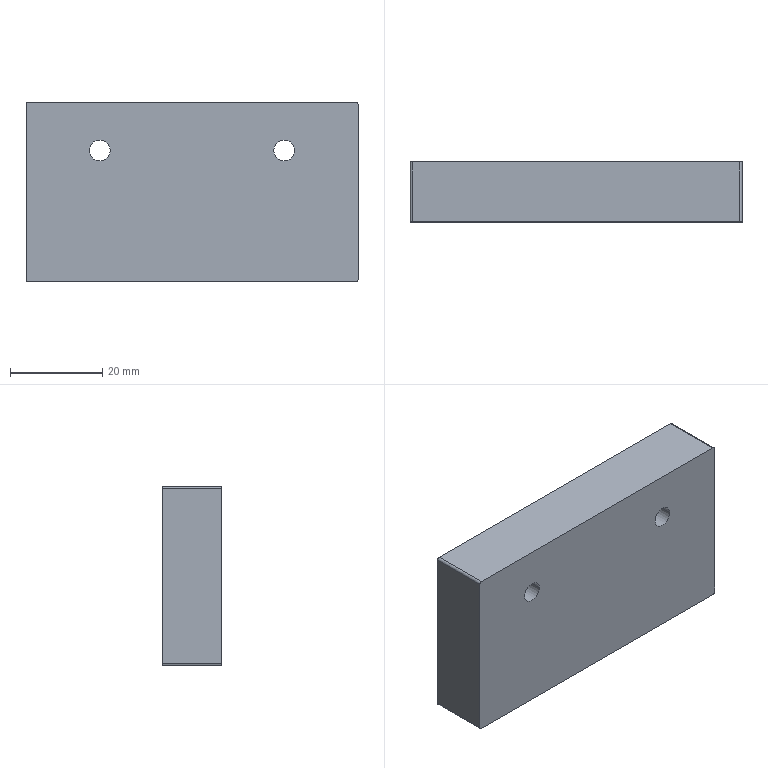Part | SolidWorks | features Extrusion 1, Fillet 1, ICE 1 | 1 solid | 14 faces | box 72 x 13 x 39 mm | volume 36088 mm3 | cylinder 8 | plane 6 | commonest cylinder face diameters 1 x4 4.5 x4
STEP:
#1=CARTESIAN_POINT('',(22.25,-6.5,28.5));
#2=VERTEX_POINT('',#1);
#3=CARTESIAN_POINT('',(17.75,-6.5,28.5));
#4=VERTEX_POINT('',#3);
#5=CARTESIAN_POINT('',(20.,-6.5,28.5));
#6=DIRECTION('',(0.,1.,0.));
#7=DIRECTION('',(-1.,0.,0.));
#8=AXIS2_PLACEMENT_3D('',#5,#6,#7);
#9=CIRCLE('',#8,2.25);
#10=EDGE_CURVE('',#2,#4,#9,.T.);
#11=ORIENTED_EDGE('',*,*,#10,.F.);
#12=CARTESIAN_POINT('',(22.25,6.5,28.5));
#13=VERTEX_POINT('',#12);
#14=CARTESIAN_POINT('',(22.25,-6.5,28.5));
#15=DIRECTION('',(0.,1.,0.));
#16=VECTOR('',#15,1000.);
#17=LINE('',#14,#16);
#18=EDGE_CURVE('',#2,#13,#17,.T.);
#19=ORIENTED_EDGE('',*,*,#18,.T.);
#20=CARTESIAN_POINT('',(17.75,6.5,28.5));
#21=VERTEX_POINT('',#20);
#22=CARTESIAN_POINT('',(20.,6.5,28.5));
#23=DIRECTION('',(0.,1.,0.));
#24=DIRECTION('',(-1.,0.,0.));
#25=AXIS2_PLACEMENT_3D('',#22,#23,#24);
#26=CIRCLE('',#25,2.25);
#27=EDGE_CURVE('',#13,#21,#26,.T.);
#28=ORIENTED_EDGE('',*,*,#27,.T.);
#29=CARTESIAN_POINT('',(17.75,-6.5,28.5));
#30=DIRECTION('',(0.,1.,0.));
#31=VECTOR('',#30,1000.);
#32=LINE('',#29,#31);
#33=EDGE_CURVE('',#4,#21,#32,.T.);
#34=ORIENTED_EDGE('',*,*,#33,.F.);
#35=EDGE_LOOP('',(#11,#19,#28,#34));
#36=FACE_OUTER_BOUND('',#35,.T.);
#37=CARTESIAN_POINT('',(20.,-6.5,28.5));
#38=DIRECTION('',(0.,1.,0.));
#39=DIRECTION('',(-1.,0.,0.));
#40=AXIS2_PLACEMENT_3D('',#37,#38,#39);
#41=CYLINDRICAL_SURFACE('',#40,2.25);
#42=ADVANCED_FACE('',(#36),#41,.F.);
#43=CARTESIAN_POINT('',(-17.75,-6.5,28.5));
#44=VERTEX_POINT('',#43);
#45=CARTESIAN_POINT('',(-22.25,-6.5,28.5));
#46=VERTEX_POINT('',#45);
#47=CARTESIAN_POINT('',(-20.,-6.5,28.5));
#48=DIRECTION('',(0.,1.,0.));
#49=DIRECTION('',(-1.,0.,0.));
#50=AXIS2_PLACEMENT_3D('',#47,#48,#49);
#51=CIRCLE('',#50,2.25);
#52=EDGE_CURVE('',#44,#46,#51,.T.);
#53=ORIENTED_EDGE('',*,*,#52,.F.);
#54=CARTESIAN_POINT('',(-17.75,6.5,28.5));
#55=VERTEX_POINT('',#54);
#56=CARTESIAN_POINT('',(-17.75,-6.5,28.5));
#57=DIRECTION('',(0.,1.,0.));
#58=VECTOR('',#57,1000.);
#59=LINE('',#56,#58);
#60=EDGE_CURVE('',#44,#55,#59,.T.);
#61=ORIENTED_EDGE('',*,*,#60,.T.);
#62=CARTESIAN_POINT('',(-22.25,6.5,28.5));
#63=VERTEX_POINT('',#62);
#64=CARTESIAN_POINT('',(-20.,6.5,28.5));
#65=DIRECTION('',(0.,1.,0.));
#66=DIRECTION('',(-1.,0.,0.));
#67=AXIS2_PLACEMENT_3D('',#64,#65,#66);
#68=CIRCLE('',#67,2.25);
#69=EDGE_CURVE('',#55,#63,#68,.T.);
#70=ORIENTED_EDGE('',*,*,#69,.T.);
#71=CARTESIAN_POINT('',(-22.25,-6.5,28.5));
#72=DIRECTION('',(0.,1.,0.));
#73=VECTOR('',#72,1000.);
#74=LINE('',#71,#73);
#75=EDGE_CURVE('',#46,#63,#74,.T.);
#76=ORIENTED_EDGE('',*,*,#75,.F.);
#77=EDGE_LOOP('',(#53,#61,#70,#76));
#78=FACE_OUTER_BOUND('',#77,.T.);
#79=CARTESIAN_POINT('',(-20.,-6.5,28.5));
#80=DIRECTION('',(0.,1.,0.));
#81=DIRECTION('',(-1.,0.,0.));
#82=AXIS2_PLACEMENT_3D('',#79,#80,#81);
#83=CYLINDRICAL_SURFACE('',#82,2.25);
#84=ADVANCED_FACE('',(#78),#83,.F.);
#85=CARTESIAN_POINT('',(-36.,-6.5,38.5));
#86=VERTEX_POINT('',#85);
#87=CARTESIAN_POINT('',(-36.,-6.5,0.5));
#88=VERTEX_POINT('',#87);
#89=CARTESIAN_POINT('',(-36.,-6.5,39.));
#90=DIRECTION('',(0.,0.,-1.));
#91=VECTOR('',#90,1000.);
#92=LINE('',#89,#91);
#93=EDGE_CURVE('',#86,#88,#92,.T.);
#94=ORIENTED_EDGE('',*,*,#93,.F.);
#95=CARTESIAN_POINT('',(-36.,6.5,38.5));
#96=VERTEX_POINT('',#95);
#97=CARTESIAN_POINT('',(-36.,6.5,38.5));
#98=DIRECTION('',(0.,1.,0.));
#99=VECTOR('',#98,1000.);
#100=LINE('',#97,#99);
#101=EDGE_CURVE('',#86,#96,#100,.T.);
#102=ORIENTED_EDGE('',*,*,#101,.T.);
#103=CARTESIAN_POINT('',(-36.,6.5,0.5));
#104=VERTEX_POINT('',#103);
#105=CARTESIAN_POINT('',(-36.,6.5,39.));
#106=DIRECTION('',(0.,0.,-1.));
#107=VECTOR('',#106,1000.);
#108=LINE('',#105,#107);
#109=EDGE_CURVE('',#96,#104,#108,.T.);
#110=ORIENTED_EDGE('',*,*,#109,.T.);
#111=CARTESIAN_POINT('',(-36.,-6.5,0.5));
#112=DIRECTION('',(0.,-1.,0.));
#113=VECTOR('',#112,1000.);
#114=LINE('',#111,#113);
#115=EDGE_CURVE('',#104,#88,#114,.T.);
#116=ORIENTED_EDGE('',*,*,#115,.T.);
#117=EDGE_LOOP('',(#94,#102,#110,#116));
#118=FACE_OUTER_BOUND('',#117,.T.);
#119=CARTESIAN_POINT('',(-36.,6.5,39.));
#120=DIRECTION('',(1.,0.,0.));
#121=DIRECTION('',(0.,0.,-1.));
#122=AXIS2_PLACEMENT_3D('',#119,#120,#121);
#123=PLANE('',#122);
#124=ADVANCED_FACE('',(#118),#123,.F.);
#125=CARTESIAN_POINT('',(20.,-6.5,28.5));
#126=DIRECTION('',(0.,1.,0.));
#127=DIRECTION('',(-1.,0.,0.));
#128=AXIS2_PLACEMENT_3D('',#125,#126,#127);
#129=CIRCLE('',#128,2.25);
#130=EDGE_CURVE('',#4,#2,#129,.T.);
#131=ORIENTED_EDGE('',*,*,#130,.T.);
#132=ORIENTED_EDGE('',*,*,#10,.T.);
#133=EDGE_LOOP('',(#131,#132));
#134=FACE_BOUND('',#133,.T.);
#135=CARTESIAN_POINT('',(-20.,-6.5,28.5));
#136=DIRECTION('',(0.,1.,0.));
#137=DIRECTION('',(-1.,0.,0.));
#138=AXIS2_PLACEMENT_3D('',#135,#136,#137);
#139=CIRCLE('',#138,2.25);
#140=EDGE_CURVE('',#46,#44,#139,.T.);
#141=ORIENTED_EDGE('',*,*,#140,.T.);
#142=ORIENTED_EDGE('',*,*,#52,.T.);
#143=EDGE_LOOP('',(#141,#142));
#144=FACE_BOUND('',#143,.T.);
#145=CARTESIAN_POINT('',(-35.5,-6.5,0.));
#146=VERTEX_POINT('',#145);
#147=CARTESIAN_POINT('',(35.5,-6.5,0.));
#148=VERTEX_POINT('',#147);
#149=CARTESIAN_POINT('',(36.,-6.5,0.));
#150=DIRECTION('',(1.,0.,0.));
#151=VECTOR('',#150,1000.);
#152=LINE('',#149,#151);
#153=EDGE_CURVE('',#146,#148,#152,.T.);
#154=ORIENTED_EDGE('',*,*,#153,.T.);
#155=CARTESIAN_POINT('',(36.,-6.5,0.5));
#156=VERTEX_POINT('',#155);
#157=CARTESIAN_POINT('',(35.5,-6.5,0.5));
#158=DIRECTION('',(0.,-1.,0.));
#159=DIRECTION('',(-1.,0.,0.));
#160=AXIS2_PLACEMENT_3D('',#157,#158,#159);
#161=CIRCLE('',#160,0.5);
#162=EDGE_CURVE('',#148,#156,#161,.T.);
#163=ORIENTED_EDGE('',*,*,#162,.T.);
#164=CARTESIAN_POINT('',(36.,-6.5,38.5));
#165=VERTEX_POINT('',#164);
#166=CARTESIAN_POINT('',(36.,-6.5,39.));
#167=DIRECTION('',(0.,0.,-1.));
#168=VECTOR('',#167,1000.);
#169=LINE('',#166,#168);
#170=EDGE_CURVE('',#165,#156,#169,.T.);
#171=ORIENTED_EDGE('',*,*,#170,.F.);
#172=CARTESIAN_POINT('',(35.5,-6.5,39.));
#173=VERTEX_POINT('',#172);
#174=CARTESIAN_POINT('',(35.5,-6.5,38.5));
#175=DIRECTION('',(0.,-1.,0.));
#176=DIRECTION('',(-1.,0.,0.));
#177=AXIS2_PLACEMENT_3D('',#174,#175,#176);
#178=CIRCLE('',#177,0.5);
#179=EDGE_CURVE('',#165,#173,#178,.T.);
#180=ORIENTED_EDGE('',*,*,#179,.T.);
#181=CARTESIAN_POINT('',(-35.5,-6.5,39.));
#182=VERTEX_POINT('',#181);
#183=CARTESIAN_POINT('',(36.,-6.5,39.));
#184=DIRECTION('',(1.,0.,0.));
#185=VECTOR('',#184,1000.);
#186=LINE('',#183,#185);
#187=EDGE_CURVE('',#182,#173,#186,.T.);
#188=ORIENTED_EDGE('',*,*,#187,.F.);
#189=CARTESIAN_POINT('',(-35.5,-6.5,38.5));
#190=DIRECTION('',(0.,-1.,0.));
#191=DIRECTION('',(-1.,0.,0.));
#192=AXIS2_PLACEMENT_3D('',#189,#190,#191);
#193=CIRCLE('',#192,0.5);
#194=EDGE_CURVE('',#182,#86,#193,.T.);
#195=ORIENTED_EDGE('',*,*,#194,.T.);
#196=ORIENTED_EDGE('',*,*,#93,.T.);
#197=CARTESIAN_POINT('',(-35.5,-6.5,0.5));
#198=DIRECTION('',(0.,-1.,0.));
#199=DIRECTION('',(-1.,0.,0.));
#200=AXIS2_PLACEMENT_3D('',#197,#198,#199);
#201=CIRCLE('',#200,0.5);
#202=EDGE_CURVE('',#88,#146,#201,.T.);
#203=ORIENTED_EDGE('',*,*,#202,.T.);
#204=EDGE_LOOP('',(#154,#163,#171,#180,#188,#195,#196,#203));
#205=FACE_OUTER_BOUND('',#204,.T.);
#206=CARTESIAN_POINT('',(36.,-6.5,39.));
#207=DIRECTION('',(0.,1.,0.));
#208=DIRECTION('',(-1.,0.,0.));
#209=AXIS2_PLACEMENT_3D('',#206,#207,#208);
#210=PLANE('',#209);
#211=ADVANCED_FACE('',(#134,#144,#205),#210,.F.);
#212=ORIENTED_EDGE('',*,*,#170,.T.);
#213=CARTESIAN_POINT('',(36.,6.5,0.5));
#214=VERTEX_POINT('',#213);
#215=CARTESIAN_POINT('',(36.,6.5,0.5));
#216=DIRECTION('',(0.,1.,0.));
#217=VECTOR('',#216,1000.);
#218=LINE('',#215,#217);
#219=EDGE_CURVE('',#156,#214,#218,.T.);
#220=ORIENTED_EDGE('',*,*,#219,.T.);
#221=CARTESIAN_POINT('',(36.,6.5,38.5));
#222=VERTEX_POINT('',#221);
#223=CARTESIAN_POINT('',(36.,6.5,39.));
#224=DIRECTION('',(0.,0.,-1.));
#225=VECTOR('',#224,1000.);
#226=LINE('',#223,#225);
#227=EDGE_CURVE('',#222,#214,#226,.T.);
#228=ORIENTED_EDGE('',*,*,#227,.F.);
#229=CARTESIAN_POINT('',(36.,6.5,38.5));
#230=DIRECTION('',(0.,-1.,0.));
#231=VECTOR('',#230,1000.);
#232=LINE('',#229,#231);
#233=EDGE_CURVE('',#222,#165,#232,.T.);
#234=ORIENTED_EDGE('',*,*,#233,.T.);
#235=EDGE_LOOP('',(#212,#220,#228,#234));
#236=FACE_OUTER_BOUND('',#235,.T.);
#237=CARTESIAN_POINT('',(36.,6.5,39.));
#238=DIRECTION('',(-1.,0.,0.));
#239=DIRECTION('',(0.,0.,1.));
#240=AXIS2_PLACEMENT_3D('',#237,#238,#239);
#241=PLANE('',#240);
#242=ADVANCED_FACE('',(#236),#241,.F.);
#243=CARTESIAN_POINT('',(20.,6.5,28.5));
#244=DIRECTION('',(0.,1.,0.));
#245=DIRECTION('',(-1.,0.,0.));
#246=AXIS2_PLACEMENT_3D('',#243,#244,#245);
#247=CIRCLE('',#246,2.25);
#248=EDGE_CURVE('',#21,#13,#247,.T.);
#249=ORIENTED_EDGE('',*,*,#248,.F.);
#250=ORIENTED_EDGE('',*,*,#27,.F.);
#251=EDGE_LOOP('',(#249,#250));
#252=FACE_BOUND('',#251,.T.);
#253=CARTESIAN_POINT('',(-20.,6.5,28.5));
#254=DIRECTION('',(0.,1.,0.));
#255=DIRECTION('',(-1.,0.,0.));
#256=AXIS2_PLACEMENT_3D('',#253,#254,#255);
#257=CIRCLE('',#256,2.25);
#258=EDGE_CURVE('',#63,#55,#257,.T.);
#259=ORIENTED_EDGE('',*,*,#258,.F.);
#260=ORIENTED_EDGE('',*,*,#69,.F.);
#261=EDGE_LOOP('',(#259,#260));
#262=FACE_BOUND('',#261,.T.);
#263=ORIENTED_EDGE('',*,*,#227,.T.);
#264=CARTESIAN_POINT('',(35.5,6.5,0.));
#265=VERTEX_POINT('',#264);
#266=CARTESIAN_POINT('',(35.5,6.5,0.5));
#267=DIRECTION('',(0.,1.,0.));
#268=DIRECTION('',(1.,0.,0.));
#269=AXIS2_PLACEMENT_3D('',#266,#267,#268);
#270=CIRCLE('',#269,0.5);
#271=EDGE_CURVE('',#214,#265,#270,.T.);
#272=ORIENTED_EDGE('',*,*,#271,.T.);
#273=CARTESIAN_POINT('',(-35.5,6.5,0.));
#274=VERTEX_POINT('',#273);
#275=CARTESIAN_POINT('',(36.,6.5,0.));
#276=DIRECTION('',(-1.,0.,0.));
#277=VECTOR('',#276,1000.);
#278=LINE('',#275,#277);
#279=EDGE_CURVE('',#265,#274,#278,.T.);
#280=ORIENTED_EDGE('',*,*,#279,.T.);
#281=CARTESIAN_POINT('',(-35.5,6.5,0.5));
#282=DIRECTION('',(0.,1.,0.));
#283=DIRECTION('',(1.,0.,0.));
#284=AXIS2_PLACEMENT_3D('',#281,#282,#283);
#285=CIRCLE('',#284,0.5);
#286=EDGE_CURVE('',#274,#104,#285,.T.);
#287=ORIENTED_EDGE('',*,*,#286,.T.);
#288=ORIENTED_EDGE('',*,*,#109,.F.);
#289=CARTESIAN_POINT('',(-35.5,6.5,39.));
#290=VERTEX_POINT('',#289);
#291=CARTESIAN_POINT('',(-35.5,6.5,38.5));
#292=DIRECTION('',(0.,1.,0.));
#293=DIRECTION('',(1.,0.,0.));
#294=AXIS2_PLACEMENT_3D('',#291,#292,#293);
#295=CIRCLE('',#294,0.5);
#296=EDGE_CURVE('',#96,#290,#295,.T.);
#297=ORIENTED_EDGE('',*,*,#296,.T.);
#298=CARTESIAN_POINT('',(35.5,6.5,39.));
#299=VERTEX_POINT('',#298);
#300=CARTESIAN_POINT('',(36.,6.5,39.));
#301=DIRECTION('',(-1.,0.,0.));
#302=VECTOR('',#301,1000.);
#303=LINE('',#300,#302);
#304=EDGE_CURVE('',#299,#290,#303,.T.);
#305=ORIENTED_EDGE('',*,*,#304,.F.);
#306=CARTESIAN_POINT('',(35.5,6.5,38.5));
#307=DIRECTION('',(0.,1.,0.));
#308=DIRECTION('',(1.,0.,0.));
#309=AXIS2_PLACEMENT_3D('',#306,#307,#308);
#310=CIRCLE('',#309,0.5);
#311=EDGE_CURVE('',#299,#222,#310,.T.);
#312=ORIENTED_EDGE('',*,*,#311,.T.);
#313=EDGE_LOOP('',(#263,#272,#280,#287,#288,#297,#305,#312));
#314=FACE_OUTER_BOUND('',#313,.T.);
#315=CARTESIAN_POINT('',(36.,6.5,39.));
#316=DIRECTION('',(0.,-1.,0.));
#317=DIRECTION('',(1.,0.,0.));
#318=AXIS2_PLACEMENT_3D('',#315,#316,#317);
#319=PLANE('',#318);
#320=ADVANCED_FACE('',(#252,#262,#314),#319,.F.);
#321=ORIENTED_EDGE('',*,*,#187,.T.);
#322=CARTESIAN_POINT('',(35.5,0.,39.));
#323=DIRECTION('',(0.,1.,0.));
#324=VECTOR('',#323,1000.);
#325=LINE('',#322,#324);
#326=EDGE_CURVE('',#173,#299,#325,.T.);
#327=ORIENTED_EDGE('',*,*,#326,.T.);
#328=ORIENTED_EDGE('',*,*,#304,.T.);
#329=CARTESIAN_POINT('',(-35.5,0.,39.));
#330=DIRECTION('',(0.,-1.,0.));
#331=VECTOR('',#330,1000.);
#332=LINE('',#329,#331);
#333=EDGE_CURVE('',#290,#182,#332,.T.);
#334=ORIENTED_EDGE('',*,*,#333,.T.);
#335=EDGE_LOOP('',(#321,#327,#328,#334));
#336=FACE_OUTER_BOUND('',#335,.T.);
#337=CARTESIAN_POINT('',(0.,0.,39.));
#338=DIRECTION('',(0.,0.,-1.));
#339=DIRECTION('',(-1.,0.,0.));
#340=AXIS2_PLACEMENT_3D('',#337,#338,#339);
#341=PLANE('',#340);
#342=ADVANCED_FACE('',(#336),#341,.F.);
#343=ORIENTED_EDGE('',*,*,#279,.F.);
#344=CARTESIAN_POINT('',(35.5,-6.5,0.));
#345=DIRECTION('',(0.,-1.,0.));
#346=VECTOR('',#345,1000.);
#347=LINE('',#344,#346);
#348=EDGE_CURVE('',#265,#148,#347,.T.);
#349=ORIENTED_EDGE('',*,*,#348,.T.);
#350=ORIENTED_EDGE('',*,*,#153,.F.);
#351=CARTESIAN_POINT('',(-35.5,6.5,0.));
#352=DIRECTION('',(0.,1.,0.));
#353=VECTOR('',#352,1000.);
#354=LINE('',#351,#353);
#355=EDGE_CURVE('',#146,#274,#354,.T.);
#356=ORIENTED_EDGE('',*,*,#355,.T.);
#357=EDGE_LOOP('',(#343,#349,#350,#356));
#358=FACE_OUTER_BOUND('',#357,.T.);
#359=CARTESIAN_POINT('',(0.,0.,0.));
#360=DIRECTION('',(0.,0.,-1.));
#361=DIRECTION('',(-1.,0.,0.));
#362=AXIS2_PLACEMENT_3D('',#359,#360,#361);
#363=PLANE('',#362);
#364=ADVANCED_FACE('',(#358),#363,.T.);
#365=ORIENTED_EDGE('',*,*,#162,.F.);
#366=ORIENTED_EDGE('',*,*,#348,.F.);
#367=ORIENTED_EDGE('',*,*,#271,.F.);
#368=ORIENTED_EDGE('',*,*,#219,.F.);
#369=EDGE_LOOP('',(#365,#366,#367,#368));
#370=FACE_OUTER_BOUND('',#369,.T.);
#371=CARTESIAN_POINT('',(35.5,6.5,0.5));
#372=DIRECTION('',(0.,-1.,0.));
#373=DIRECTION('',(0.,0.,-1.));
#374=AXIS2_PLACEMENT_3D('',#371,#372,#373);
#375=CYLINDRICAL_SURFACE('',#374,0.5);
#376=ADVANCED_FACE('',(#370),#375,.T.);
#377=ORIENTED_EDGE('',*,*,#179,.F.);
#378=ORIENTED_EDGE('',*,*,#233,.F.);
#379=ORIENTED_EDGE('',*,*,#311,.F.);
#380=ORIENTED_EDGE('',*,*,#326,.F.);
#381=EDGE_LOOP('',(#377,#378,#379,#380));
#382=FACE_OUTER_BOUND('',#381,.T.);
#383=CARTESIAN_POINT('',(35.5,0.,38.5));
#384=DIRECTION('',(0.,1.,0.));
#385=DIRECTION('',(0.,0.,1.));
#386=AXIS2_PLACEMENT_3D('',#383,#384,#385);
#387=CYLINDRICAL_SURFACE('',#386,0.5);
#388=ADVANCED_FACE('',(#382),#387,.T.);
#389=ORIENTED_EDGE('',*,*,#296,.F.);
#390=ORIENTED_EDGE('',*,*,#101,.F.);
#391=ORIENTED_EDGE('',*,*,#194,.F.);
#392=ORIENTED_EDGE('',*,*,#333,.F.);
#393=EDGE_LOOP('',(#389,#390,#391,#392));
#394=FACE_OUTER_BOUND('',#393,.T.);
#395=CARTESIAN_POINT('',(-35.5,0.,38.5));
#396=DIRECTION('',(0.,-1.,0.));
#397=DIRECTION('',(0.,0.,-1.));
#398=AXIS2_PLACEMENT_3D('',#395,#396,#397);
#399=CYLINDRICAL_SURFACE('',#398,0.5);
#400=ADVANCED_FACE('',(#394),#399,.T.);
#401=ORIENTED_EDGE('',*,*,#286,.F.);
#402=ORIENTED_EDGE('',*,*,#355,.F.);
#403=ORIENTED_EDGE('',*,*,#202,.F.);
#404=ORIENTED_EDGE('',*,*,#115,.F.);
#405=EDGE_LOOP('',(#401,#402,#403,#404));
#406=FACE_OUTER_BOUND('',#405,.T.);
#407=CARTESIAN_POINT('',(-35.5,6.5,0.5));
#408=DIRECTION('',(0.,1.,0.));
#409=DIRECTION('',(0.,0.,1.));
#410=AXIS2_PLACEMENT_3D('',#407,#408,#409);
#411=CYLINDRICAL_SURFACE('',#410,0.5);
#412=ADVANCED_FACE('',(#406),#411,.T.);
#413=ORIENTED_EDGE('',*,*,#60,.F.);
#414=ORIENTED_EDGE('',*,*,#140,.F.);
#415=ORIENTED_EDGE('',*,*,#75,.T.);
#416=ORIENTED_EDGE('',*,*,#258,.T.);
#417=EDGE_LOOP('',(#413,#414,#415,#416));
#418=FACE_OUTER_BOUND('',#417,.T.);
#419=CARTESIAN_POINT('',(-20.,-6.5,28.5));
#420=DIRECTION('',(0.,1.,0.));
#421=DIRECTION('',(-1.,0.,0.));
#422=AXIS2_PLACEMENT_3D('',#419,#420,#421);
#423=CYLINDRICAL_SURFACE('',#422,2.25);
#424=ADVANCED_FACE('',(#418),#423,.F.);
#425=ORIENTED_EDGE('',*,*,#18,.F.);
#426=ORIENTED_EDGE('',*,*,#130,.F.);
#427=ORIENTED_EDGE('',*,*,#33,.T.);
#428=ORIENTED_EDGE('',*,*,#248,.T.);
#429=EDGE_LOOP('',(#425,#426,#427,#428));
#430=FACE_OUTER_BOUND('',#429,.T.);
#431=CARTESIAN_POINT('',(20.,-6.5,28.5));
#432=DIRECTION('',(0.,1.,0.));
#433=DIRECTION('',(-1.,0.,0.));
#434=AXIS2_PLACEMENT_3D('',#431,#432,#433);
#435=CYLINDRICAL_SURFACE('',#434,2.25);
#436=ADVANCED_FACE('',(#430),#435,.F.);
#437=CLOSED_SHELL('',(#42,#84,#124,#211,#242,#320,#342,#364,#376,#388,#400,#412,#424,#436));
#438=MANIFOLD_SOLID_BREP('',#437);
#439=CARTESIAN_POINT('',(0.,0.,0.));
#440=DIRECTION('',(0.,0.,1.));
#441=DIRECTION('',(1.,0.,0.));
#442=AXIS2_PLACEMENT_3D('',#439,#440,#441);
#443=(LENGTH_UNIT()NAMED_UNIT(*)SI_UNIT(.MILLI.,.METRE.));
#444=UNCERTAINTY_MEASURE_WITH_UNIT(LENGTH_MEASURE(0.00001),#443,'','');
#445=(NAMED_UNIT(*)PLANE_ANGLE_UNIT()SI_UNIT($,.RADIAN.));
#446=(NAMED_UNIT(*)SI_UNIT($,.STERADIAN.)SOLID_ANGLE_UNIT());
#447=(GEOMETRIC_REPRESENTATION_CONTEXT(3)GLOBAL_UNCERTAINTY_ASSIGNED_CONTEXT((#444))GLOBAL_UNIT_ASSIGNED_CONTEXT((#443,#445,#446))REPRESENTATION_CONTEXT('',''));
#448=ADVANCED_BREP_SHAPE_REPRESENTATION('',(#438,#442),#447);